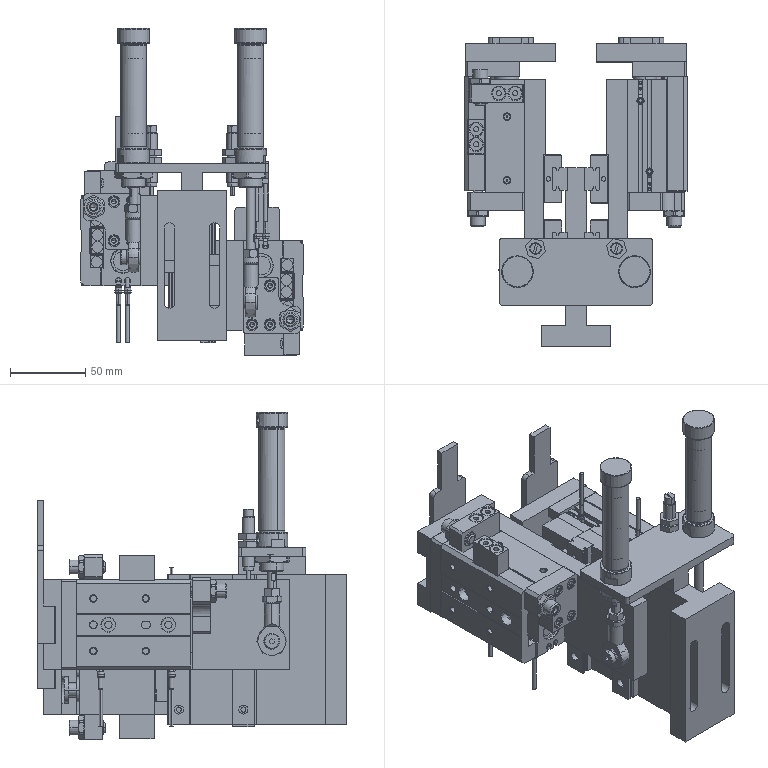Part | SolidWorks | 37 solids | 2796 faces | box 148 x 205.5 x 218 mm | volume 1082273 mm3 | plane 1318 | cylinder 934 | cone 430 | spline 106 | torus 8 | commonest cylinder face diameters 4.134 x64 6 x52 16 x42 4.2 x40 7.5 x40 0.4 x32